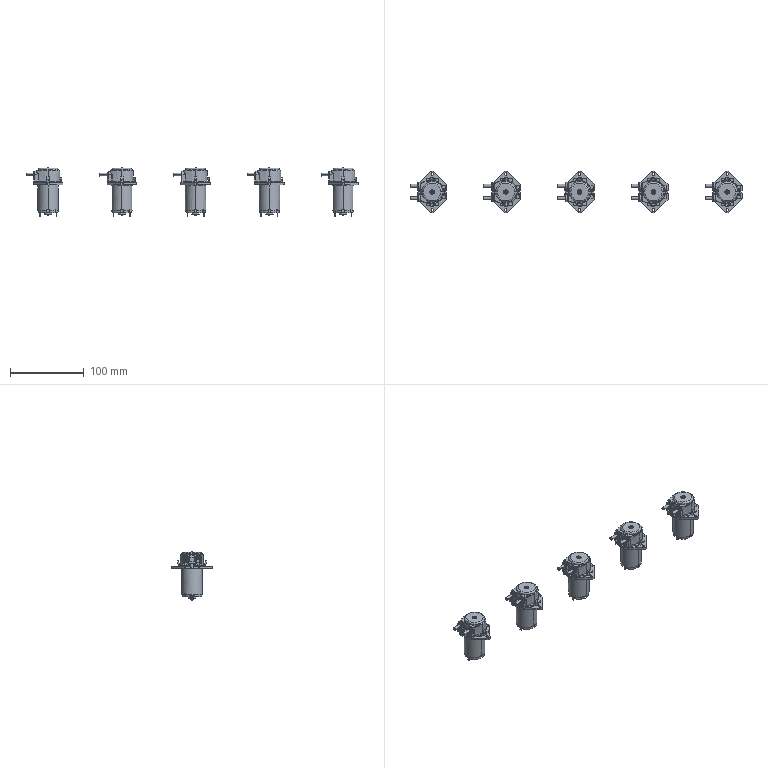Part | SolidWorks | 60 solids | 4435 faces | volume 191920 mm3 | plane 2125 | cylinder 1595 | torus 385 | cone 210 | sphere 80 | spline 40 | commonest cylinder face diameters 0.2 x140 2 x130 2.515 x130 0.5 x120 1.799 x120 1 x100